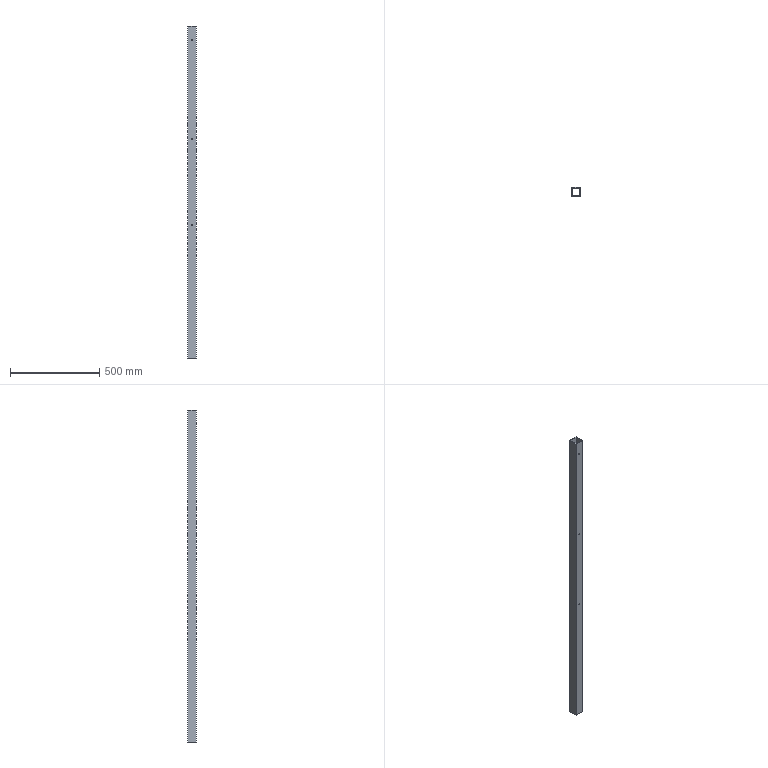Part | NX | features solid 2 | 1 solid | 16 faces | box 50 x 50 x 1856 mm | volume 1669976 mm3 | plane 10 | cylinder 6 | commonest cylinder face diameters 6 x6
STEP:
#1=CARTESIAN_POINT('',(605.,475.,180.));
#2=VERTEX_POINT('',#1);
#3=CARTESIAN_POINT('',(605.,480.,180.));
#4=VERTEX_POINT('',#3);
#5=CARTESIAN_POINT('',(605.,2286.381,180.));
#6=DIRECTION('',(0.,-1.,0.));
#7=VECTOR('',#6,1000.);
#8=LINE('',#5,#7);
#9=EDGE_CURVE('',#2,#4,#8,.F.);
#10=ORIENTED_EDGE('',*,*,#9,.T.);
#11=CARTESIAN_POINT('',(605.,480.,186.));
#12=VERTEX_POINT('',#11);
#13=CARTESIAN_POINT('',(605.,480.,183.));
#14=DIRECTION('',(0.,1.,0.));
#15=DIRECTION('',(0.,0.,-1.));
#16=AXIS2_PLACEMENT_3D('',#13,#14,#15);
#17=CIRCLE('',#16,3.);
#18=EDGE_CURVE('',#4,#12,#17,.T.);
#19=ORIENTED_EDGE('',*,*,#18,.T.);
#20=CARTESIAN_POINT('',(605.,475.,186.));
#21=VERTEX_POINT('',#20);
#22=CARTESIAN_POINT('',(605.,2286.381,186.));
#23=DIRECTION('',(0.,-1.,0.));
#24=VECTOR('',#23,1000.);
#25=LINE('',#22,#24);
#26=EDGE_CURVE('',#12,#21,#25,.T.);
#27=ORIENTED_EDGE('',*,*,#26,.T.);
#28=CARTESIAN_POINT('',(605.,475.,183.));
#29=DIRECTION('',(0.,-1.,0.));
#30=DIRECTION('',(0.,0.,1.));
#31=AXIS2_PLACEMENT_3D('',#28,#29,#30);
#32=CIRCLE('',#31,3.);
#33=EDGE_CURVE('',#21,#2,#32,.T.);
#34=ORIENTED_EDGE('',*,*,#33,.T.);
#35=EDGE_LOOP('',(#10,#19,#27,#34));
#36=FACE_BOUND('',#35,.T.);
#37=CARTESIAN_POINT('',(605.,2286.381,183.));
#38=DIRECTION('',(0.,-1.,0.));
#39=DIRECTION('',(0.,0.,1.));
#40=AXIS2_PLACEMENT_3D('',#37,#38,#39);
#41=CYLINDRICAL_SURFACE('',#40,3.);
#42=ADVANCED_FACE('',(#36),#41,.F.);
#43=CARTESIAN_POINT('',(605.,480.,660.));
#44=VERTEX_POINT('',#43);
#45=CARTESIAN_POINT('',(605.,475.,660.));
#46=VERTEX_POINT('',#45);
#47=CARTESIAN_POINT('',(605.,2286.381,660.));
#48=DIRECTION('',(0.,-1.,0.));
#49=VECTOR('',#48,1000.);
#50=LINE('',#47,#49);
#51=EDGE_CURVE('',#44,#46,#50,.T.);
#52=ORIENTED_EDGE('',*,*,#51,.F.);
#53=CARTESIAN_POINT('',(605.,480.,666.));
#54=VERTEX_POINT('',#53);
#55=CARTESIAN_POINT('',(605.,480.,663.));
#56=DIRECTION('',(0.,1.,0.));
#57=DIRECTION('',(0.,0.,-1.));
#58=AXIS2_PLACEMENT_3D('',#55,#56,#57);
#59=CIRCLE('',#58,3.);
#60=EDGE_CURVE('',#44,#54,#59,.T.);
#61=ORIENTED_EDGE('',*,*,#60,.T.);
#62=CARTESIAN_POINT('',(605.,475.,666.));
#63=VERTEX_POINT('',#62);
#64=CARTESIAN_POINT('',(605.,2286.381,666.));
#65=DIRECTION('',(0.,-1.,0.));
#66=VECTOR('',#65,1000.);
#67=LINE('',#64,#66);
#68=EDGE_CURVE('',#63,#54,#67,.F.);
#69=ORIENTED_EDGE('',*,*,#68,.F.);
#70=CARTESIAN_POINT('',(605.,475.,663.));
#71=DIRECTION('',(0.,-1.,0.));
#72=DIRECTION('',(0.,0.,1.));
#73=AXIS2_PLACEMENT_3D('',#70,#71,#72);
#74=CIRCLE('',#73,3.);
#75=EDGE_CURVE('',#63,#46,#74,.T.);
#76=ORIENTED_EDGE('',*,*,#75,.T.);
#77=EDGE_LOOP('',(#52,#61,#69,#76));
#78=FACE_BOUND('',#77,.T.);
#79=CARTESIAN_POINT('',(605.,2286.381,663.));
#80=DIRECTION('',(0.,-1.,0.));
#81=DIRECTION('',(0.,0.,1.));
#82=AXIS2_PLACEMENT_3D('',#79,#80,#81);
#83=CYLINDRICAL_SURFACE('',#82,3.);
#84=ADVANCED_FACE('',(#78),#83,.F.);
#85=CARTESIAN_POINT('',(605.,480.,1210.));
#86=VERTEX_POINT('',#85);
#87=CARTESIAN_POINT('',(605.,475.,1210.));
#88=VERTEX_POINT('',#87);
#89=CARTESIAN_POINT('',(605.,2286.381,1210.));
#90=DIRECTION('',(0.,-1.,0.));
#91=VECTOR('',#90,1000.);
#92=LINE('',#89,#91);
#93=EDGE_CURVE('',#86,#88,#92,.T.);
#94=ORIENTED_EDGE('',*,*,#93,.F.);
#95=CARTESIAN_POINT('',(605.,480.,1216.));
#96=VERTEX_POINT('',#95);
#97=CARTESIAN_POINT('',(605.,480.,1213.));
#98=DIRECTION('',(0.,1.,0.));
#99=DIRECTION('',(0.,0.,-1.));
#100=AXIS2_PLACEMENT_3D('',#97,#98,#99);
#101=CIRCLE('',#100,3.);
#102=EDGE_CURVE('',#86,#96,#101,.T.);
#103=ORIENTED_EDGE('',*,*,#102,.T.);
#104=CARTESIAN_POINT('',(605.,475.,1216.));
#105=VERTEX_POINT('',#104);
#106=CARTESIAN_POINT('',(605.,2286.381,1216.));
#107=DIRECTION('',(0.,-1.,0.));
#108=VECTOR('',#107,1000.);
#109=LINE('',#106,#108);
#110=EDGE_CURVE('',#105,#96,#109,.F.);
#111=ORIENTED_EDGE('',*,*,#110,.F.);
#112=CARTESIAN_POINT('',(605.,475.,1213.));
#113=DIRECTION('',(0.,-1.,0.));
#114=DIRECTION('',(0.,0.,1.));
#115=AXIS2_PLACEMENT_3D('',#112,#113,#114);
#116=CIRCLE('',#115,3.);
#117=EDGE_CURVE('',#105,#88,#116,.T.);
#118=ORIENTED_EDGE('',*,*,#117,.T.);
#119=EDGE_LOOP('',(#94,#103,#111,#118));
#120=FACE_BOUND('',#119,.T.);
#121=CARTESIAN_POINT('',(605.,2286.381,1213.));
#122=DIRECTION('',(0.,-1.,0.));
#123=DIRECTION('',(0.,0.,1.));
#124=AXIS2_PLACEMENT_3D('',#121,#122,#123);
#125=CYLINDRICAL_SURFACE('',#124,3.);
#126=ADVANCED_FACE('',(#120),#125,.F.);
#127=CARTESIAN_POINT('',(580.,525.,-563.));
#128=VERTEX_POINT('',#127);
#129=CARTESIAN_POINT('',(580.,525.,1293.));
#130=VERTEX_POINT('',#129);
#131=CARTESIAN_POINT('',(580.,525.,-447.));
#132=DIRECTION('',(0.,0.,1.));
#133=VECTOR('',#132,1000.);
#134=LINE('',#131,#133);
#135=EDGE_CURVE('',#128,#130,#134,.T.);
#136=ORIENTED_EDGE('',*,*,#135,.T.);
#137=CARTESIAN_POINT('',(630.,525.,1293.));
#138=VERTEX_POINT('',#137);
#139=CARTESIAN_POINT('',(580.,525.,1293.));
#140=DIRECTION('',(-1.,0.,0.));
#141=VECTOR('',#140,1000.);
#142=LINE('',#139,#141);
#143=EDGE_CURVE('',#138,#130,#142,.T.);
#144=ORIENTED_EDGE('',*,*,#143,.F.);
#145=CARTESIAN_POINT('',(630.,525.,-563.));
#146=VERTEX_POINT('',#145);
#147=CARTESIAN_POINT('',(630.,525.,-447.));
#148=DIRECTION('',(0.,0.,-1.));
#149=VECTOR('',#148,1000.);
#150=LINE('',#147,#149);
#151=EDGE_CURVE('',#138,#146,#150,.T.);
#152=ORIENTED_EDGE('',*,*,#151,.T.);
#153=CARTESIAN_POINT('',(580.,525.,-563.));
#154=DIRECTION('',(-1.,0.,0.));
#155=VECTOR('',#154,1000.);
#156=LINE('',#153,#155);
#157=EDGE_CURVE('',#146,#128,#156,.T.);
#158=ORIENTED_EDGE('',*,*,#157,.T.);
#159=EDGE_LOOP('',(#136,#144,#152,#158));
#160=FACE_BOUND('',#159,.T.);
#161=CARTESIAN_POINT('',(580.,525.,-447.));
#162=DIRECTION('',(0.,-1.,0.));
#163=DIRECTION('',(-1.,0.,0.));
#164=AXIS2_PLACEMENT_3D('',#161,#162,#163);
#165=PLANE('',#164);
#166=ADVANCED_FACE('',(#160),#165,.F.);
#167=CARTESIAN_POINT('',(585.,520.,1293.));
#168=VERTEX_POINT('',#167);
#169=CARTESIAN_POINT('',(625.,520.,1293.));
#170=VERTEX_POINT('',#169);
#171=CARTESIAN_POINT('',(630.,520.,1293.));
#172=DIRECTION('',(1.,0.,0.));
#173=VECTOR('',#172,1000.);
#174=LINE('',#171,#173);
#175=EDGE_CURVE('',#168,#170,#174,.T.);
#176=ORIENTED_EDGE('',*,*,#175,.F.);
#177=CARTESIAN_POINT('',(585.,520.,-563.));
#178=VERTEX_POINT('',#177);
#179=CARTESIAN_POINT('',(585.,520.,-447.));
#180=DIRECTION('',(0.,0.,1.));
#181=VECTOR('',#180,1000.);
#182=LINE('',#179,#181);
#183=EDGE_CURVE('',#178,#168,#182,.T.);
#184=ORIENTED_EDGE('',*,*,#183,.F.);
#185=CARTESIAN_POINT('',(625.,520.,-563.));
#186=VERTEX_POINT('',#185);
#187=CARTESIAN_POINT('',(630.,520.,-563.));
#188=DIRECTION('',(1.,0.,0.));
#189=VECTOR('',#188,1000.);
#190=LINE('',#187,#189);
#191=EDGE_CURVE('',#178,#186,#190,.T.);
#192=ORIENTED_EDGE('',*,*,#191,.T.);
#193=CARTESIAN_POINT('',(625.,520.,-447.));
#194=DIRECTION('',(0.,0.,-1.));
#195=VECTOR('',#194,1000.);
#196=LINE('',#193,#195);
#197=EDGE_CURVE('',#170,#186,#196,.T.);
#198=ORIENTED_EDGE('',*,*,#197,.F.);
#199=EDGE_LOOP('',(#176,#184,#192,#198));
#200=FACE_BOUND('',#199,.T.);
#201=CARTESIAN_POINT('',(585.,520.,-447.));
#202=DIRECTION('',(0.,-1.,0.));
#203=DIRECTION('',(-1.,0.,0.));
#204=AXIS2_PLACEMENT_3D('',#201,#202,#203);
#205=PLANE('',#204);
#206=ADVANCED_FACE('',(#200),#205,.T.);
#207=CARTESIAN_POINT('',(580.,475.,-563.));
#208=VERTEX_POINT('',#207);
#209=CARTESIAN_POINT('',(580.,475.,1293.));
#210=VERTEX_POINT('',#209);
#211=CARTESIAN_POINT('',(580.,475.,1293.));
#212=DIRECTION('',(0.,0.,1.));
#213=VECTOR('',#212,1000.);
#214=LINE('',#211,#213);
#215=EDGE_CURVE('',#208,#210,#214,.T.);
#216=ORIENTED_EDGE('',*,*,#215,.T.);
#217=CARTESIAN_POINT('',(580.,475.,1293.));
#218=DIRECTION('',(0.,-1.,0.));
#219=VECTOR('',#218,1000.);
#220=LINE('',#217,#219);
#221=EDGE_CURVE('',#130,#210,#220,.T.);
#222=ORIENTED_EDGE('',*,*,#221,.F.);
#223=ORIENTED_EDGE('',*,*,#135,.F.);
#224=CARTESIAN_POINT('',(580.,475.,-563.));
#225=DIRECTION('',(0.,-1.,0.));
#226=VECTOR('',#225,1000.);
#227=LINE('',#224,#226);
#228=EDGE_CURVE('',#128,#208,#227,.T.);
#229=ORIENTED_EDGE('',*,*,#228,.T.);
#230=EDGE_LOOP('',(#216,#222,#223,#229));
#231=FACE_BOUND('',#230,.T.);
#232=CARTESIAN_POINT('',(580.,475.,1293.));
#233=DIRECTION('',(1.,0.,0.));
#234=DIRECTION('',(0.,-1.,0.));
#235=AXIS2_PLACEMENT_3D('',#232,#233,#234);
#236=PLANE('',#235);
#237=ADVANCED_FACE('',(#231),#236,.F.);
#238=ORIENTED_EDGE('',*,*,#151,.F.);
#239=CARTESIAN_POINT('',(630.,475.,1293.));
#240=VERTEX_POINT('',#239);
#241=CARTESIAN_POINT('',(630.,475.,1293.));
#242=DIRECTION('',(0.,1.,0.));
#243=VECTOR('',#242,1000.);
#244=LINE('',#241,#243);
#245=EDGE_CURVE('',#240,#138,#244,.T.);
#246=ORIENTED_EDGE('',*,*,#245,.F.);
#247=CARTESIAN_POINT('',(630.,475.,-563.));
#248=VERTEX_POINT('',#247);
#249=CARTESIAN_POINT('',(630.,475.,-447.));
#250=DIRECTION('',(0.,0.,-1.));
#251=VECTOR('',#250,1000.);
#252=LINE('',#249,#251);
#253=EDGE_CURVE('',#240,#248,#252,.T.);
#254=ORIENTED_EDGE('',*,*,#253,.T.);
#255=CARTESIAN_POINT('',(630.,475.,-563.));
#256=DIRECTION('',(0.,1.,0.));
#257=VECTOR('',#256,1000.);
#258=LINE('',#255,#257);
#259=EDGE_CURVE('',#248,#146,#258,.T.);
#260=ORIENTED_EDGE('',*,*,#259,.T.);
#261=EDGE_LOOP('',(#238,#246,#254,#260));
#262=FACE_BOUND('',#261,.T.);
#263=CARTESIAN_POINT('',(630.,475.,-447.));
#264=DIRECTION('',(-1.,0.,0.));
#265=DIRECTION('',(0.,0.,1.));
#266=AXIS2_PLACEMENT_3D('',#263,#264,#265);
#267=PLANE('',#266);
#268=ADVANCED_FACE('',(#262),#267,.F.);
#269=CARTESIAN_POINT('',(625.,480.,-563.));
#270=VERTEX_POINT('',#269);
#271=CARTESIAN_POINT('',(625.,475.,-563.));
#272=DIRECTION('',(0.,-1.,0.));
#273=VECTOR('',#272,1000.);
#274=LINE('',#271,#273);
#275=EDGE_CURVE('',#186,#270,#274,.T.);
#276=ORIENTED_EDGE('',*,*,#275,.F.);
#277=ORIENTED_EDGE('',*,*,#191,.F.);
#278=CARTESIAN_POINT('',(585.,480.,-563.));
#279=VERTEX_POINT('',#278);
#280=CARTESIAN_POINT('',(585.,475.,-563.));
#281=DIRECTION('',(0.,1.,0.));
#282=VECTOR('',#281,1000.);
#283=LINE('',#280,#282);
#284=EDGE_CURVE('',#279,#178,#283,.T.);
#285=ORIENTED_EDGE('',*,*,#284,.F.);
#286=CARTESIAN_POINT('',(630.,480.,-563.));
#287=DIRECTION('',(-1.,0.,0.));
#288=VECTOR('',#287,1000.);
#289=LINE('',#286,#288);
#290=EDGE_CURVE('',#270,#279,#289,.T.);
#291=ORIENTED_EDGE('',*,*,#290,.F.);
#292=EDGE_LOOP('',(#276,#277,#285,#291));
#293=FACE_BOUND('',#292,.T.);
#294=ORIENTED_EDGE('',*,*,#228,.F.);
#295=ORIENTED_EDGE('',*,*,#157,.F.);
#296=ORIENTED_EDGE('',*,*,#259,.F.);
#297=CARTESIAN_POINT('',(630.,475.,-563.));
#298=DIRECTION('',(-1.,0.,0.));
#299=VECTOR('',#298,1000.);
#300=LINE('',#297,#299);
#301=EDGE_CURVE('',#248,#208,#300,.T.);
#302=ORIENTED_EDGE('',*,*,#301,.T.);
#303=EDGE_LOOP('',(#294,#295,#296,#302));
#304=FACE_BOUND('',#303,.T.);
#305=CARTESIAN_POINT('',(630.,475.,-563.));
#306=DIRECTION('',(0.,0.,1.));
#307=DIRECTION('',(0.,-1.,0.));
#308=AXIS2_PLACEMENT_3D('',#305,#306,#307);
#309=PLANE('',#308);
#310=ADVANCED_FACE('',(#293,#304),#309,.F.);
#311=CARTESIAN_POINT('',(585.,480.,1293.));
#312=VERTEX_POINT('',#311);
#313=CARTESIAN_POINT('',(585.,475.,1293.));
#314=DIRECTION('',(0.,1.,0.));
#315=VECTOR('',#314,1000.);
#316=LINE('',#313,#315);
#317=EDGE_CURVE('',#312,#168,#316,.T.);
#318=ORIENTED_EDGE('',*,*,#317,.F.);
#319=CARTESIAN_POINT('',(585.,480.,1293.));
#320=DIRECTION('',(0.,0.,1.));
#321=VECTOR('',#320,1000.);
#322=LINE('',#319,#321);
#323=EDGE_CURVE('',#279,#312,#322,.T.);
#324=ORIENTED_EDGE('',*,*,#323,.F.);
#325=ORIENTED_EDGE('',*,*,#284,.T.);
#326=ORIENTED_EDGE('',*,*,#183,.T.);
#327=EDGE_LOOP('',(#318,#324,#325,#326));
#328=FACE_BOUND('',#327,.T.);
#329=CARTESIAN_POINT('',(585.,480.,1293.));
#330=DIRECTION('',(1.,0.,0.));
#331=DIRECTION('',(0.,-1.,0.));
#332=AXIS2_PLACEMENT_3D('',#329,#330,#331);
#333=PLANE('',#332);
#334=ADVANCED_FACE('',(#328),#333,.T.);
#335=ORIENTED_EDGE('',*,*,#317,.T.);
#336=ORIENTED_EDGE('',*,*,#175,.T.);
#337=CARTESIAN_POINT('',(625.,480.,1293.));
#338=VERTEX_POINT('',#337);
#339=CARTESIAN_POINT('',(625.,520.,1293.));
#340=DIRECTION('',(0.,1.,0.));
#341=VECTOR('',#340,1000.);
#342=LINE('',#339,#341);
#343=EDGE_CURVE('',#338,#170,#342,.T.);
#344=ORIENTED_EDGE('',*,*,#343,.F.);
#345=CARTESIAN_POINT('',(625.,480.,1293.));
#346=DIRECTION('',(1.,0.,0.));
#347=VECTOR('',#346,1000.);
#348=LINE('',#345,#347);
#349=EDGE_CURVE('',#312,#338,#348,.T.);
#350=ORIENTED_EDGE('',*,*,#349,.F.);
#351=EDGE_LOOP('',(#335,#336,#344,#350));
#352=FACE_BOUND('',#351,.T.);
#353=ORIENTED_EDGE('',*,*,#143,.T.);
#354=ORIENTED_EDGE('',*,*,#221,.T.);
#355=CARTESIAN_POINT('',(630.,475.,1293.));
#356=DIRECTION('',(1.,0.,0.));
#357=VECTOR('',#356,1000.);
#358=LINE('',#355,#357);
#359=EDGE_CURVE('',#210,#240,#358,.T.);
#360=ORIENTED_EDGE('',*,*,#359,.T.);
#361=ORIENTED_EDGE('',*,*,#245,.T.);
#362=EDGE_LOOP('',(#353,#354,#360,#361));
#363=FACE_BOUND('',#362,.T.);
#364=CARTESIAN_POINT('',(630.,475.,1293.));
#365=DIRECTION('',(0.,0.,1.));
#366=DIRECTION('',(0.,-1.,0.));
#367=AXIS2_PLACEMENT_3D('',#364,#365,#366);
#368=PLANE('',#367);
#369=ADVANCED_FACE('',(#352,#363),#368,.T.);
#370=ORIENTED_EDGE('',*,*,#343,.T.);
#371=ORIENTED_EDGE('',*,*,#197,.T.);
#372=ORIENTED_EDGE('',*,*,#275,.T.);
#373=CARTESIAN_POINT('',(625.,480.,-447.));
#374=DIRECTION('',(0.,0.,-1.));
#375=VECTOR('',#374,1000.);
#376=LINE('',#373,#375);
#377=EDGE_CURVE('',#338,#270,#376,.T.);
#378=ORIENTED_EDGE('',*,*,#377,.F.);
#379=EDGE_LOOP('',(#370,#371,#372,#378));
#380=FACE_BOUND('',#379,.T.);
#381=CARTESIAN_POINT('',(625.,520.,-447.));
#382=DIRECTION('',(-1.,0.,0.));
#383=DIRECTION('',(0.,0.,1.));
#384=AXIS2_PLACEMENT_3D('',#381,#382,#383);
#385=PLANE('',#384);
#386=ADVANCED_FACE('',(#380),#385,.T.);
#387=ORIENTED_EDGE('',*,*,#117,.F.);
#388=CARTESIAN_POINT('',(605.,475.,1213.));
#389=DIRECTION('',(0.,-1.,0.));
#390=DIRECTION('',(0.,0.,1.));
#391=AXIS2_PLACEMENT_3D('',#388,#389,#390);
#392=CIRCLE('',#391,3.);
#393=EDGE_CURVE('',#88,#105,#392,.T.);
#394=ORIENTED_EDGE('',*,*,#393,.F.);
#395=EDGE_LOOP('',(#387,#394));
#396=FACE_BOUND('',#395,.T.);
#397=ORIENTED_EDGE('',*,*,#75,.F.);
#398=CARTESIAN_POINT('',(605.,475.,663.));
#399=DIRECTION('',(0.,-1.,0.));
#400=DIRECTION('',(0.,0.,1.));
#401=AXIS2_PLACEMENT_3D('',#398,#399,#400);
#402=CIRCLE('',#401,3.);
#403=EDGE_CURVE('',#46,#63,#402,.T.);
#404=ORIENTED_EDGE('',*,*,#403,.F.);
#405=EDGE_LOOP('',(#397,#404));
#406=FACE_BOUND('',#405,.T.);
#407=ORIENTED_EDGE('',*,*,#33,.F.);
#408=CARTESIAN_POINT('',(605.,475.,183.));
#409=DIRECTION('',(0.,-1.,0.));
#410=DIRECTION('',(0.,0.,1.));
#411=AXIS2_PLACEMENT_3D('',#408,#409,#410);
#412=CIRCLE('',#411,3.);
#413=EDGE_CURVE('',#2,#21,#412,.T.);
#414=ORIENTED_EDGE('',*,*,#413,.F.);
#415=EDGE_LOOP('',(#407,#414));
#416=FACE_BOUND('',#415,.T.);
#417=ORIENTED_EDGE('',*,*,#253,.F.);
#418=ORIENTED_EDGE('',*,*,#359,.F.);
#419=ORIENTED_EDGE('',*,*,#215,.F.);
#420=ORIENTED_EDGE('',*,*,#301,.F.);
#421=EDGE_LOOP('',(#417,#418,#419,#420));
#422=FACE_BOUND('',#421,.T.);
#423=CARTESIAN_POINT('',(630.,475.,-447.));
#424=DIRECTION('',(0.,1.,0.));
#425=DIRECTION('',(1.,0.,0.));
#426=AXIS2_PLACEMENT_3D('',#423,#424,#425);
#427=PLANE('',#426);
#428=ADVANCED_FACE('',(#396,#406,#416,#422),#427,.F.);
#429=CARTESIAN_POINT('',(605.,480.,1213.));
#430=DIRECTION('',(0.,1.,0.));
#431=DIRECTION('',(0.,0.,-1.));
#432=AXIS2_PLACEMENT_3D('',#429,#430,#431);
#433=CIRCLE('',#432,3.);
#434=EDGE_CURVE('',#96,#86,#433,.T.);
#435=ORIENTED_EDGE('',*,*,#434,.F.);
#436=ORIENTED_EDGE('',*,*,#102,.F.);
#437=EDGE_LOOP('',(#435,#436));
#438=FACE_BOUND('',#437,.T.);
#439=CARTESIAN_POINT('',(605.,480.,663.));
#440=DIRECTION('',(0.,1.,0.));
#441=DIRECTION('',(0.,0.,-1.));
#442=AXIS2_PLACEMENT_3D('',#439,#440,#441);
#443=CIRCLE('',#442,3.);
#444=EDGE_CURVE('',#54,#44,#443,.T.);
#445=ORIENTED_EDGE('',*,*,#444,.F.);
#446=ORIENTED_EDGE('',*,*,#60,.F.);
#447=EDGE_LOOP('',(#445,#446));
#448=FACE_BOUND('',#447,.T.);
#449=CARTESIAN_POINT('',(605.,480.,183.));
#450=DIRECTION('',(0.,1.,0.));
#451=DIRECTION('',(0.,0.,-1.));
#452=AXIS2_PLACEMENT_3D('',#449,#450,#451);
#453=CIRCLE('',#452,3.);
#454=EDGE_CURVE('',#12,#4,#453,.T.);
#455=ORIENTED_EDGE('',*,*,#454,.F.);
#456=ORIENTED_EDGE('',*,*,#18,.F.);
#457=EDGE_LOOP('',(#455,#456));
#458=FACE_BOUND('',#457,.T.);
#459=ORIENTED_EDGE('',*,*,#349,.T.);
#460=ORIENTED_EDGE('',*,*,#377,.T.);
#461=ORIENTED_EDGE('',*,*,#290,.T.);
#462=ORIENTED_EDGE('',*,*,#323,.T.);
#463=EDGE_LOOP('',(#459,#460,#461,#462));
#464=FACE_BOUND('',#463,.T.);
#465=CARTESIAN_POINT('',(625.,480.,1293.));
#466=DIRECTION('',(0.,1.,0.));
#467=DIRECTION('',(1.,0.,0.));
#468=AXIS2_PLACEMENT_3D('',#465,#466,#467);
#469=PLANE('',#468);
#470=ADVANCED_FACE('',(#438,#448,#458,#464),#469,.T.);
#471=ORIENTED_EDGE('',*,*,#434,.T.);
#472=ORIENTED_EDGE('',*,*,#93,.T.);
#473=ORIENTED_EDGE('',*,*,#393,.T.);
#474=ORIENTED_EDGE('',*,*,#110,.T.);
#475=EDGE_LOOP('',(#471,#472,#473,#474));
#476=FACE_BOUND('',#475,.T.);
#477=CARTESIAN_POINT('',(605.,2286.381,1213.));
#478=DIRECTION('',(0.,-1.,0.));
#479=DIRECTION('',(0.,0.,1.));
#480=AXIS2_PLACEMENT_3D('',#477,#478,#479);
#481=CYLINDRICAL_SURFACE('',#480,3.);
#482=ADVANCED_FACE('',(#476),#481,.F.);
#483=ORIENTED_EDGE('',*,*,#444,.T.);
#484=ORIENTED_EDGE('',*,*,#51,.T.);
#485=ORIENTED_EDGE('',*,*,#403,.T.);
#486=ORIENTED_EDGE('',*,*,#68,.T.);
#487=EDGE_LOOP('',(#483,#484,#485,#486));
#488=FACE_BOUND('',#487,.T.);
#489=CARTESIAN_POINT('',(605.,2286.381,663.));
#490=DIRECTION('',(0.,-1.,0.));
#491=DIRECTION('',(0.,0.,1.));
#492=AXIS2_PLACEMENT_3D('',#489,#490,#491);
#493=CYLINDRICAL_SURFACE('',#492,3.);
#494=ADVANCED_FACE('',(#488),#493,.F.);
#495=ORIENTED_EDGE('',*,*,#454,.T.);
#496=ORIENTED_EDGE('',*,*,#9,.F.);
#497=ORIENTED_EDGE('',*,*,#413,.T.);
#498=ORIENTED_EDGE('',*,*,#26,.F.);
#499=EDGE_LOOP('',(#495,#496,#497,#498));
#500=FACE_BOUND('',#499,.T.);
#501=CARTESIAN_POINT('',(605.,2286.381,183.));
#502=DIRECTION('',(0.,-1.,0.));
#503=DIRECTION('',(0.,0.,1.));
#504=AXIS2_PLACEMENT_3D('',#501,#502,#503);
#505=CYLINDRICAL_SURFACE('',#504,3.);
#506=ADVANCED_FACE('',(#500),#505,.F.);
#507=CLOSED_SHELL('',(#42,#84,#126,#166,#206,#237,#268,#310,#334,#369,#386,#428,#470,#482,#494,#506));
#508=MANIFOLD_SOLID_BREP('',#507);
#509=(LENGTH_UNIT()NAMED_UNIT(*)SI_UNIT(.MILLI.,.METRE.));
#510=UNCERTAINTY_MEASURE_WITH_UNIT(LENGTH_MEASURE(0.00001),#509,'','');
#511=(NAMED_UNIT(*)PLANE_ANGLE_UNIT()SI_UNIT($,.RADIAN.));
#512=(NAMED_UNIT(*)SI_UNIT($,.STERADIAN.)SOLID_ANGLE_UNIT());
#513=(GEOMETRIC_REPRESENTATION_CONTEXT(3)GLOBAL_UNCERTAINTY_ASSIGNED_CONTEXT((#510))GLOBAL_UNIT_ASSIGNED_CONTEXT((#509,#511,#512))REPRESENTATION_CONTEXT('',''));
#514=ADVANCED_BREP_SHAPE_REPRESENTATION('',(#508),#513);